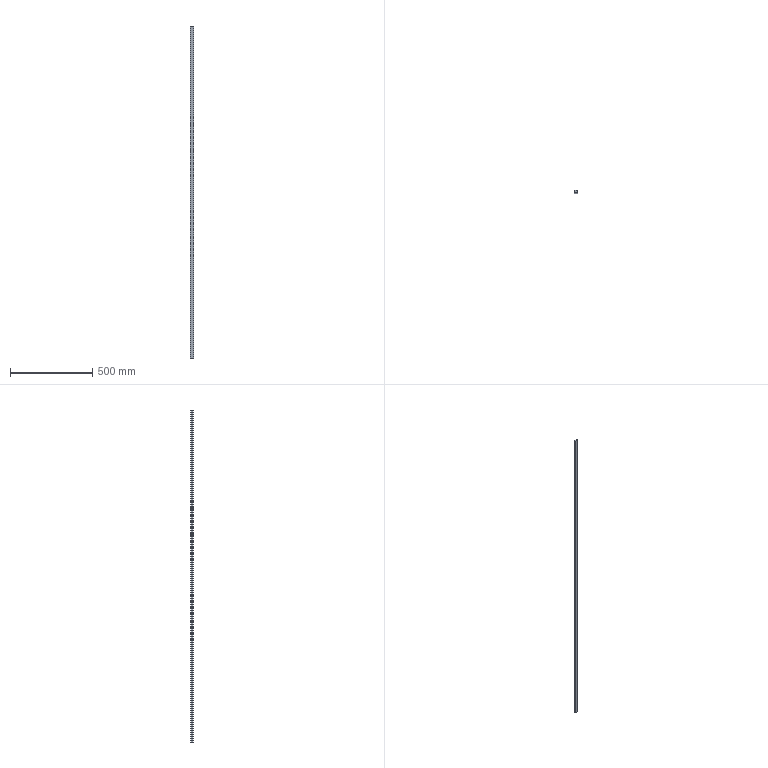Part | STEP file | rail_SX2RZ28_280 | 1 solid | 15 faces | box 20 x 15.5 x 2022 mm | volume 581693 mm3 | plane 10 | cylinder 5 | commonest cylinder face diameters 5 x3 3 x2
STEP:
#1=CARTESIAN_POINT('',(0.,0.,0.));
#2=DIRECTION('',(0.,0.,1.));
#3=DIRECTION('',(1.,0.,0.));
#4=AXIS2_PLACEMENT_3D('',#1,#2,#3);
#5=CARTESIAN_POINT('',(9.062,11.498,1.));
#6=VERTEX_POINT('',#5);
#7=CARTESIAN_POINT('',(9.062,11.498,-2020.5));
#8=VERTEX_POINT('',#7);
#9=CARTESIAN_POINT('',(9.062,11.498,1.));
#10=DIRECTION('',(0.,0.,-1.));
#11=VECTOR('',#10,1.);
#12=LINE('',#9,#11);
#13=CARTESIAN_POINT('',(10.,9.18,1.));
#14=DIRECTION('',(0.,0.,-1.));
#15=DIRECTION('',(-1.,0.,0.));
#16=AXIS2_PLACEMENT_3D('',#13,#14,#15);
#17=CYLINDRICAL_SURFACE('',#16,2.5);
#18=CARTESIAN_POINT('',(1.186,0.));
#19=DIRECTION('',(0.,1.));
#20=VECTOR('',#19,1.);
#21=LINE('',#18,#20);
#22=(GEOMETRIC_REPRESENTATION_CONTEXT(2)PARAMETRIC_REPRESENTATION_CONTEXT()REPRESENTATION_CONTEXT('',''));
#23=DEFINITIONAL_REPRESENTATION('',(#21),#22);
#24=PCURVE('',#17,#23);
#25=CARTESIAN_POINT('',(8.5,12.888,1.));
#26=DIRECTION('',(0.,0.,-1.));
#27=DIRECTION('',(-1.,0.,0.));
#28=AXIS2_PLACEMENT_3D('',#25,#26,#27);
#29=CYLINDRICAL_SURFACE('',#28,1.5);
#30=CARTESIAN_POINT('',(4.328,0.));
#31=DIRECTION('',(0.,1.));
#32=VECTOR('',#31,1.);
#33=LINE('',#30,#32);
#34=(GEOMETRIC_REPRESENTATION_CONTEXT(2)PARAMETRIC_REPRESENTATION_CONTEXT()REPRESENTATION_CONTEXT('',''));
#35=DEFINITIONAL_REPRESENTATION('',(#33),#34);
#36=PCURVE('',#29,#35);
#37=SURFACE_CURVE('',#12,(#24,#36),.PCURVE_S1.);
#38=EDGE_CURVE('',#6,#8,#37,.T.);
#39=ORIENTED_EDGE('',*,*,#38,.T.);
#40=CARTESIAN_POINT('',(7.5,9.18,-2020.5));
#41=VERTEX_POINT('',#40);
#42=CARTESIAN_POINT('',(10.,9.18,-2020.5));
#43=DIRECTION('',(0.,0.,-1.));
#44=DIRECTION('',(-1.,0.,0.));
#45=AXIS2_PLACEMENT_3D('',#42,#43,#44);
#46=CIRCLE('',#45,2.5);
#47=CARTESIAN_POINT('',(0.,2021.5));
#48=DIRECTION('',(1.,0.));
#49=VECTOR('',#48,1.);
#50=LINE('',#47,#49);
#51=(GEOMETRIC_REPRESENTATION_CONTEXT(2)PARAMETRIC_REPRESENTATION_CONTEXT()REPRESENTATION_CONTEXT('',''));
#52=DEFINITIONAL_REPRESENTATION('',(#50),#51);
#53=PCURVE('',#17,#52);
#54=CARTESIAN_POINT('',(10.,9.18,-2020.5));
#55=DIRECTION('',(0.,0.,-1.));
#56=DIRECTION('',(-1.,0.,0.));
#57=AXIS2_PLACEMENT_3D('',#54,#55,#56);
#58=PLANE('',#57);
#59=CARTESIAN_POINT('',(0.,0.));
#60=DIRECTION('',(1.,0.));
#61=AXIS2_PLACEMENT_2D('',#59,#60);
#62=CIRCLE('',#61,2.5);
#63=(GEOMETRIC_REPRESENTATION_CONTEXT(2)PARAMETRIC_REPRESENTATION_CONTEXT()REPRESENTATION_CONTEXT('',''));
#64=DEFINITIONAL_REPRESENTATION('',(#62),#63);
#65=PCURVE('',#58,#64);
#66=SURFACE_CURVE('',#46,(#53,#65),.PCURVE_S1.);
#67=EDGE_CURVE('',#41,#8,#66,.T.);
#68=ORIENTED_EDGE('',*,*,#67,.F.);
#69=CARTESIAN_POINT('',(7.5,9.18,1.));
#70=VERTEX_POINT('',#69);
#71=CARTESIAN_POINT('',(7.5,9.18,1.));
#72=DIRECTION('',(0.,0.,-1.));
#73=VECTOR('',#72,1.);
#74=LINE('',#71,#73);
#75=CARTESIAN_POINT('',(0.,0.));
#76=DIRECTION('',(0.,1.));
#77=VECTOR('',#76,1.);
#78=LINE('',#75,#77);
#79=(GEOMETRIC_REPRESENTATION_CONTEXT(2)PARAMETRIC_REPRESENTATION_CONTEXT()REPRESENTATION_CONTEXT('',''));
#80=DEFINITIONAL_REPRESENTATION('',(#78),#79);
#81=PCURVE('',#17,#80);
#82=CARTESIAN_POINT('',(10.,9.18,1.));
#83=DIRECTION('',(0.,0.,-1.));
#84=DIRECTION('',(-1.,0.,0.));
#85=AXIS2_PLACEMENT_3D('',#82,#83,#84);
#86=CYLINDRICAL_SURFACE('',#85,2.5);
#87=CARTESIAN_POINT('',(6.283,0.));
#88=DIRECTION('',(0.,1.));
#89=VECTOR('',#88,1.);
#90=LINE('',#87,#89);
#91=(GEOMETRIC_REPRESENTATION_CONTEXT(2)PARAMETRIC_REPRESENTATION_CONTEXT()REPRESENTATION_CONTEXT('',''));
#92=DEFINITIONAL_REPRESENTATION('',(#90),#91);
#93=PCURVE('',#86,#92);
#94=SURFACE_CURVE('',#74,(#81,#93),.PCURVE_S1.);
#95=EDGE_CURVE('',#70,#41,#94,.T.);
#96=ORIENTED_EDGE('',*,*,#95,.F.);
#97=CARTESIAN_POINT('',(10.,9.18,1.));
#98=DIRECTION('',(0.,0.,-1.));
#99=DIRECTION('',(-1.,0.,0.));
#100=AXIS2_PLACEMENT_3D('',#97,#98,#99);
#101=CIRCLE('',#100,2.5);
#102=CARTESIAN_POINT('',(0.,0.));
#103=DIRECTION('',(1.,0.));
#104=VECTOR('',#103,1.);
#105=LINE('',#102,#104);
#106=(GEOMETRIC_REPRESENTATION_CONTEXT(2)PARAMETRIC_REPRESENTATION_CONTEXT()REPRESENTATION_CONTEXT('',''));
#107=DEFINITIONAL_REPRESENTATION('',(#105),#106);
#108=PCURVE('',#17,#107);
#109=CARTESIAN_POINT('',(10.,9.18,1.));
#110=DIRECTION('',(0.,0.,-1.));
#111=DIRECTION('',(-1.,0.,0.));
#112=AXIS2_PLACEMENT_3D('',#109,#110,#111);
#113=PLANE('',#112);
#114=CARTESIAN_POINT('',(0.,0.));
#115=DIRECTION('',(1.,0.));
#116=AXIS2_PLACEMENT_2D('',#114,#115);
#117=CIRCLE('',#116,2.5);
#118=(GEOMETRIC_REPRESENTATION_CONTEXT(2)PARAMETRIC_REPRESENTATION_CONTEXT()REPRESENTATION_CONTEXT('',''));
#119=DEFINITIONAL_REPRESENTATION('',(#117),#118);
#120=PCURVE('',#113,#119);
#121=SURFACE_CURVE('',#101,(#108,#120),.PCURVE_S1.);
#122=EDGE_CURVE('',#70,#6,#121,.T.);
#123=ORIENTED_EDGE('',*,*,#122,.T.);
#124=EDGE_LOOP('',(#39,#68,#96,#123));
#125=FACE_BOUND('',#124,.F.);
#126=ADVANCED_FACE('',(#125),#17,.F.);
#127=CARTESIAN_POINT('',(-10.,6.68,1.));
#128=VERTEX_POINT('',#127);
#129=CARTESIAN_POINT('',(-10.,6.68,-2020.5));
#130=VERTEX_POINT('',#129);
#131=CARTESIAN_POINT('',(-10.,6.68,1.));
#132=DIRECTION('',(0.,0.,-1.));
#133=VECTOR('',#132,1.);
#134=LINE('',#131,#133);
#135=CARTESIAN_POINT('',(-10.,6.68,1.));
#136=DIRECTION('',(1.,0.,0.));
#137=DIRECTION('',(0.,0.,-1.));
#138=AXIS2_PLACEMENT_3D('',#135,#136,#137);
#139=PLANE('',#138);
#140=CARTESIAN_POINT('',(0.,0.));
#141=DIRECTION('',(1.,0.));
#142=VECTOR('',#141,1.);
#143=LINE('',#140,#142);
#144=(GEOMETRIC_REPRESENTATION_CONTEXT(2)PARAMETRIC_REPRESENTATION_CONTEXT()REPRESENTATION_CONTEXT('',''));
#145=DEFINITIONAL_REPRESENTATION('',(#143),#144);
#146=PCURVE('',#139,#145);
#147=CARTESIAN_POINT('',(-10.,9.18,1.));
#148=DIRECTION('',(0.,0.,-1.));
#149=DIRECTION('',(-1.,0.,0.));
#150=AXIS2_PLACEMENT_3D('',#147,#148,#149);
#151=CYLINDRICAL_SURFACE('',#150,2.5);
#152=CARTESIAN_POINT('',(4.712,0.));
#153=DIRECTION('',(0.,1.));
#154=VECTOR('',#153,1.);
#155=LINE('',#152,#154);
#156=(GEOMETRIC_REPRESENTATION_CONTEXT(2)PARAMETRIC_REPRESENTATION_CONTEXT()REPRESENTATION_CONTEXT('',''));
#157=DEFINITIONAL_REPRESENTATION('',(#155),#156);
#158=PCURVE('',#151,#157);
#159=SURFACE_CURVE('',#134,(#146,#158),.PCURVE_S1.);
#160=EDGE_CURVE('',#128,#130,#159,.T.);
#161=ORIENTED_EDGE('',*,*,#160,.T.);
#162=CARTESIAN_POINT('',(-10.,0.,-2020.5));
#163=VERTEX_POINT('',#162);
#164=CARTESIAN_POINT('',(-10.,6.68,-2020.5));
#165=DIRECTION('',(0.,-1.,0.));
#166=VECTOR('',#165,1.);
#167=LINE('',#164,#166);
#168=CARTESIAN_POINT('',(2021.5,0.));
#169=DIRECTION('',(0.,-1.));
#170=VECTOR('',#169,1.);
#171=LINE('',#168,#170);
#172=(GEOMETRIC_REPRESENTATION_CONTEXT(2)PARAMETRIC_REPRESENTATION_CONTEXT()REPRESENTATION_CONTEXT('',''));
#173=DEFINITIONAL_REPRESENTATION('',(#171),#172);
#174=PCURVE('',#139,#173);
#175=CARTESIAN_POINT('',(20.,-2.5));
#176=DIRECTION('',(0.,-1.));
#177=VECTOR('',#176,1.);
#178=LINE('',#175,#177);
#179=(GEOMETRIC_REPRESENTATION_CONTEXT(2)PARAMETRIC_REPRESENTATION_CONTEXT()REPRESENTATION_CONTEXT('',''));
#180=DEFINITIONAL_REPRESENTATION('',(#178),#179);
#181=PCURVE('',#58,#180);
#182=SURFACE_CURVE('',#167,(#174,#181),.PCURVE_S1.);
#183=EDGE_CURVE('',#130,#163,#182,.T.);
#184=ORIENTED_EDGE('',*,*,#183,.T.);
#185=CARTESIAN_POINT('',(-10.,0.,1.));
#186=VERTEX_POINT('',#185);
#187=CARTESIAN_POINT('',(-10.,0.,1.));
#188=DIRECTION('',(0.,0.,-1.));
#189=VECTOR('',#188,1.);
#190=LINE('',#187,#189);
#191=CARTESIAN_POINT('',(0.,-6.68));
#192=DIRECTION('',(1.,0.));
#193=VECTOR('',#192,1.);
#194=LINE('',#191,#193);
#195=(GEOMETRIC_REPRESENTATION_CONTEXT(2)PARAMETRIC_REPRESENTATION_CONTEXT()REPRESENTATION_CONTEXT('',''));
#196=DEFINITIONAL_REPRESENTATION('',(#194),#195);
#197=PCURVE('',#139,#196);
#198=CARTESIAN_POINT('',(-10.,0.,1.));
#199=DIRECTION('',(0.,1.,0.));
#200=DIRECTION('',(0.,0.,1.));
#201=AXIS2_PLACEMENT_3D('',#198,#199,#200);
#202=PLANE('',#201);
#203=CARTESIAN_POINT('',(0.,0.));
#204=DIRECTION('',(-1.,0.));
#205=VECTOR('',#204,1.);
#206=LINE('',#203,#205);
#207=(GEOMETRIC_REPRESENTATION_CONTEXT(2)PARAMETRIC_REPRESENTATION_CONTEXT()REPRESENTATION_CONTEXT('',''));
#208=DEFINITIONAL_REPRESENTATION('',(#206),#207);
#209=PCURVE('',#202,#208);
#210=SURFACE_CURVE('',#190,(#197,#209),.PCURVE_S1.);
#211=EDGE_CURVE('',#186,#163,#210,.T.);
#212=ORIENTED_EDGE('',*,*,#211,.F.);
#213=CARTESIAN_POINT('',(-10.,6.68,1.));
#214=DIRECTION('',(0.,-1.,0.));
#215=VECTOR('',#214,1.);
#216=LINE('',#213,#215);
#217=CARTESIAN_POINT('',(0.,0.));
#218=DIRECTION('',(0.,-1.));
#219=VECTOR('',#218,1.);
#220=LINE('',#217,#219);
#221=(GEOMETRIC_REPRESENTATION_CONTEXT(2)PARAMETRIC_REPRESENTATION_CONTEXT()REPRESENTATION_CONTEXT('',''));
#222=DEFINITIONAL_REPRESENTATION('',(#220),#221);
#223=PCURVE('',#139,#222);
#224=CARTESIAN_POINT('',(20.,-2.5));
#225=DIRECTION('',(0.,-1.));
#226=VECTOR('',#225,1.);
#227=LINE('',#224,#226);
#228=(GEOMETRIC_REPRESENTATION_CONTEXT(2)PARAMETRIC_REPRESENTATION_CONTEXT()REPRESENTATION_CONTEXT('',''));
#229=DEFINITIONAL_REPRESENTATION('',(#227),#228);
#230=PCURVE('',#113,#229);
#231=SURFACE_CURVE('',#216,(#223,#230),.PCURVE_S1.);
#232=EDGE_CURVE('',#128,#186,#231,.T.);
#233=ORIENTED_EDGE('',*,*,#232,.F.);
#234=EDGE_LOOP('',(#161,#184,#212,#233));
#235=FACE_BOUND('',#234,.T.);
#236=ADVANCED_FACE('',(#235),#139,.F.);
#237=ORIENTED_EDGE('',*,*,#211,.T.);
#238=CARTESIAN_POINT('',(10.,0.,-2020.5));
#239=VERTEX_POINT('',#238);
#240=CARTESIAN_POINT('',(-10.,0.,-2020.5));
#241=DIRECTION('',(1.,0.,0.));
#242=VECTOR('',#241,1.);
#243=LINE('',#240,#242);
#244=CARTESIAN_POINT('',(-2021.5,0.));
#245=DIRECTION('',(0.,1.));
#246=VECTOR('',#245,1.);
#247=LINE('',#244,#246);
#248=(GEOMETRIC_REPRESENTATION_CONTEXT(2)PARAMETRIC_REPRESENTATION_CONTEXT()REPRESENTATION_CONTEXT('',''));
#249=DEFINITIONAL_REPRESENTATION('',(#247),#248);
#250=PCURVE('',#202,#249);
#251=CARTESIAN_POINT('',(20.,-9.18));
#252=DIRECTION('',(-1.,0.));
#253=VECTOR('',#252,1.);
#254=LINE('',#251,#253);
#255=(GEOMETRIC_REPRESENTATION_CONTEXT(2)PARAMETRIC_REPRESENTATION_CONTEXT()REPRESENTATION_CONTEXT('',''));
#256=DEFINITIONAL_REPRESENTATION('',(#254),#255);
#257=PCURVE('',#58,#256);
#258=SURFACE_CURVE('',#243,(#250,#257),.PCURVE_S1.);
#259=EDGE_CURVE('',#163,#239,#258,.T.);
#260=ORIENTED_EDGE('',*,*,#259,.T.);
#261=CARTESIAN_POINT('',(10.,0.,1.));
#262=VERTEX_POINT('',#261);
#263=CARTESIAN_POINT('',(10.,0.,1.));
#264=DIRECTION('',(0.,0.,-1.));
#265=VECTOR('',#264,1.);
#266=LINE('',#263,#265);
#267=CARTESIAN_POINT('',(0.,20.));
#268=DIRECTION('',(-1.,0.));
#269=VECTOR('',#268,1.);
#270=LINE('',#267,#269);
#271=(GEOMETRIC_REPRESENTATION_CONTEXT(2)PARAMETRIC_REPRESENTATION_CONTEXT()REPRESENTATION_CONTEXT('',''));
#272=DEFINITIONAL_REPRESENTATION('',(#270),#271);
#273=PCURVE('',#202,#272);
#274=CARTESIAN_POINT('',(10.,0.,1.));
#275=DIRECTION('',(-1.,0.,0.));
#276=DIRECTION('',(0.,0.,1.));
#277=AXIS2_PLACEMENT_3D('',#274,#275,#276);
#278=PLANE('',#277);
#279=CARTESIAN_POINT('',(0.,0.));
#280=DIRECTION('',(-1.,0.));
#281=VECTOR('',#280,1.);
#282=LINE('',#279,#281);
#283=(GEOMETRIC_REPRESENTATION_CONTEXT(2)PARAMETRIC_REPRESENTATION_CONTEXT()REPRESENTATION_CONTEXT('',''));
#284=DEFINITIONAL_REPRESENTATION('',(#282),#283);
#285=PCURVE('',#278,#284);
#286=SURFACE_CURVE('',#266,(#273,#285),.PCURVE_S1.);
#287=EDGE_CURVE('',#262,#239,#286,.T.);
#288=ORIENTED_EDGE('',*,*,#287,.F.);
#289=CARTESIAN_POINT('',(-10.,0.,1.));
#290=DIRECTION('',(1.,0.,0.));
#291=VECTOR('',#290,1.);
#292=LINE('',#289,#291);
#293=CARTESIAN_POINT('',(0.,0.));
#294=DIRECTION('',(0.,1.));
#295=VECTOR('',#294,1.);
#296=LINE('',#293,#295);
#297=(GEOMETRIC_REPRESENTATION_CONTEXT(2)PARAMETRIC_REPRESENTATION_CONTEXT()REPRESENTATION_CONTEXT('',''));
#298=DEFINITIONAL_REPRESENTATION('',(#296),#297);
#299=PCURVE('',#202,#298);
#300=CARTESIAN_POINT('',(20.,-9.18));
#301=DIRECTION('',(-1.,0.));
#302=VECTOR('',#301,1.);
#303=LINE('',#300,#302);
#304=(GEOMETRIC_REPRESENTATION_CONTEXT(2)PARAMETRIC_REPRESENTATION_CONTEXT()REPRESENTATION_CONTEXT('',''));
#305=DEFINITIONAL_REPRESENTATION('',(#303),#304);
#306=PCURVE('',#113,#305);
#307=SURFACE_CURVE('',#292,(#299,#306),.PCURVE_S1.);
#308=EDGE_CURVE('',#186,#262,#307,.T.);
#309=ORIENTED_EDGE('',*,*,#308,.F.);
#310=EDGE_LOOP('',(#237,#260,#288,#309));
#311=FACE_BOUND('',#310,.T.);
#312=ADVANCED_FACE('',(#311),#202,.F.);
#313=ORIENTED_EDGE('',*,*,#287,.T.);
#314=CARTESIAN_POINT('',(10.,6.68,-2020.5));
#315=VERTEX_POINT('',#314);
#316=CARTESIAN_POINT('',(10.,0.,-2020.5));
#317=DIRECTION('',(0.,1.,0.));
#318=VECTOR('',#317,1.);
#319=LINE('',#316,#318);
#320=CARTESIAN_POINT('',(-2021.5,0.));
#321=DIRECTION('',(0.,1.));
#322=VECTOR('',#321,1.);
#323=LINE('',#320,#322);
#324=(GEOMETRIC_REPRESENTATION_CONTEXT(2)PARAMETRIC_REPRESENTATION_CONTEXT()REPRESENTATION_CONTEXT('',''));
#325=DEFINITIONAL_REPRESENTATION('',(#323),#324);
#326=PCURVE('',#278,#325);
#327=CARTESIAN_POINT('',(0.,-9.18));
#328=DIRECTION('',(0.,1.));
#329=VECTOR('',#328,1.);
#330=LINE('',#327,#329);
#331=(GEOMETRIC_REPRESENTATION_CONTEXT(2)PARAMETRIC_REPRESENTATION_CONTEXT()REPRESENTATION_CONTEXT('',''));
#332=DEFINITIONAL_REPRESENTATION('',(#330),#331);
#333=PCURVE('',#58,#332);
#334=SURFACE_CURVE('',#319,(#326,#333),.PCURVE_S1.);
#335=EDGE_CURVE('',#239,#315,#334,.T.);
#336=ORIENTED_EDGE('',*,*,#335,.T.);
#337=CARTESIAN_POINT('',(10.,6.68,1.));
#338=VERTEX_POINT('',#337);
#339=CARTESIAN_POINT('',(10.,6.68,1.));
#340=DIRECTION('',(0.,0.,-1.));
#341=VECTOR('',#340,1.);
#342=LINE('',#339,#341);
#343=CARTESIAN_POINT('',(0.,6.68));
#344=DIRECTION('',(-1.,0.));
#345=VECTOR('',#344,1.);
#346=LINE('',#343,#345);
#347=(GEOMETRIC_REPRESENTATION_CONTEXT(2)PARAMETRIC_REPRESENTATION_CONTEXT()REPRESENTATION_CONTEXT('',''));
#348=DEFINITIONAL_REPRESENTATION('',(#346),#347);
#349=PCURVE('',#278,#348);
#350=CARTESIAN_POINT('',(4.712,0.));
#351=DIRECTION('',(0.,1.));
#352=VECTOR('',#351,1.);
#353=LINE('',#350,#352);
#354=(GEOMETRIC_REPRESENTATION_CONTEXT(2)PARAMETRIC_REPRESENTATION_CONTEXT()REPRESENTATION_CONTEXT('',''));
#355=DEFINITIONAL_REPRESENTATION('',(#353),#354);
#356=PCURVE('',#86,#355);
#357=SURFACE_CURVE('',#342,(#349,#356),.PCURVE_S1.);
#358=EDGE_CURVE('',#338,#315,#357,.T.);
#359=ORIENTED_EDGE('',*,*,#358,.F.);
#360=CARTESIAN_POINT('',(10.,0.,1.));
#361=DIRECTION('',(0.,1.,0.));
#362=VECTOR('',#361,1.);
#363=LINE('',#360,#362);
#364=CARTESIAN_POINT('',(0.,0.));
#365=DIRECTION('',(0.,1.));
#366=VECTOR('',#365,1.);
#367=LINE('',#364,#366);
#368=(GEOMETRIC_REPRESENTATION_CONTEXT(2)PARAMETRIC_REPRESENTATION_CONTEXT()REPRESENTATION_CONTEXT('',''));
#369=DEFINITIONAL_REPRESENTATION('',(#367),#368);
#370=PCURVE('',#278,#369);
#371=CARTESIAN_POINT('',(0.,-9.18));
#372=DIRECTION('',(0.,1.));
#373=VECTOR('',#372,1.);
#374=LINE('',#371,#373);
#375=(GEOMETRIC_REPRESENTATION_CONTEXT(2)PARAMETRIC_REPRESENTATION_CONTEXT()REPRESENTATION_CONTEXT('',''));
#376=DEFINITIONAL_REPRESENTATION('',(#374),#375);
#377=PCURVE('',#113,#376);
#378=SURFACE_CURVE('',#363,(#370,#377),.PCURVE_S1.);
#379=EDGE_CURVE('',#262,#338,#378,.T.);
#380=ORIENTED_EDGE('',*,*,#379,.F.);
#381=EDGE_LOOP('',(#313,#336,#359,#380));
#382=FACE_BOUND('',#381,.T.);
#383=ADVANCED_FACE('',(#382),#278,.F.);
#384=CARTESIAN_POINT('',(10.,9.18,-2020.5));
#385=DIRECTION('',(0.,0.,-1.));
#386=DIRECTION('',(-1.,0.,0.));
#387=AXIS2_PLACEMENT_3D('',#384,#385,#386);
#388=CIRCLE('',#387,2.5);
#389=CARTESIAN_POINT('',(0.,2021.5));
#390=DIRECTION('',(1.,0.));
#391=VECTOR('',#390,1.);
#392=LINE('',#389,#391);
#393=(GEOMETRIC_REPRESENTATION_CONTEXT(2)PARAMETRIC_REPRESENTATION_CONTEXT()REPRESENTATION_CONTEXT('',''));
#394=DEFINITIONAL_REPRESENTATION('',(#392),#393);
#395=PCURVE('',#86,#394);
#396=CARTESIAN_POINT('',(0.,0.));
#397=DIRECTION('',(1.,0.));
#398=AXIS2_PLACEMENT_2D('',#396,#397);
#399=CIRCLE('',#398,2.5);
#400=(GEOMETRIC_REPRESENTATION_CONTEXT(2)PARAMETRIC_REPRESENTATION_CONTEXT()REPRESENTATION_CONTEXT('',''));
#401=DEFINITIONAL_REPRESENTATION('',(#399),#400);
#402=PCURVE('',#58,#401);
#403=SURFACE_CURVE('',#388,(#395,#402),.PCURVE_S1.);
#404=EDGE_CURVE('',#315,#41,#403,.T.);
#405=ORIENTED_EDGE('',*,*,#404,.F.);
#406=ORIENTED_EDGE('',*,*,#358,.F.);
#407=CARTESIAN_POINT('',(10.,9.18,1.));
#408=DIRECTION('',(0.,0.,-1.));
#409=DIRECTION('',(-1.,0.,0.));
#410=AXIS2_PLACEMENT_3D('',#407,#408,#409);
#411=CIRCLE('',#410,2.5);
#412=CARTESIAN_POINT('',(0.,0.));
#413=DIRECTION('',(1.,0.));
#414=VECTOR('',#413,1.);
#415=LINE('',#412,#414);
#416=(GEOMETRIC_REPRESENTATION_CONTEXT(2)PARAMETRIC_REPRESENTATION_CONTEXT()REPRESENTATION_CONTEXT('',''));
#417=DEFINITIONAL_REPRESENTATION('',(#415),#416);
#418=PCURVE('',#86,#417);
#419=CARTESIAN_POINT('',(0.,0.));
#420=DIRECTION('',(1.,0.));
#421=AXIS2_PLACEMENT_2D('',#419,#420);
#422=CIRCLE('',#421,2.5);
#423=(GEOMETRIC_REPRESENTATION_CONTEXT(2)PARAMETRIC_REPRESENTATION_CONTEXT()REPRESENTATION_CONTEXT('',''));
#424=DEFINITIONAL_REPRESENTATION('',(#422),#423);
#425=PCURVE('',#113,#424);
#426=SURFACE_CURVE('',#411,(#418,#425),.PCURVE_S1.);
#427=EDGE_CURVE('',#338,#70,#426,.T.);
#428=ORIENTED_EDGE('',*,*,#427,.T.);
#429=ORIENTED_EDGE('',*,*,#95,.T.);
#430=EDGE_LOOP('',(#405,#406,#428,#429));
#431=FACE_BOUND('',#430,.F.);
#432=ADVANCED_FACE('',(#431),#86,.F.);
#433=ORIENTED_EDGE('',*,*,#38,.T.);
#434=CARTESIAN_POINT('',(10.,12.888,-2020.5));
#435=VERTEX_POINT('',#434);
#436=CARTESIAN_POINT('',(8.5,12.888,-2020.5));
#437=DIRECTION('',(0.,0.,1.));
#438=DIRECTION('',(1.,0.,0.));
#439=AXIS2_PLACEMENT_3D('',#436,#437,#438);
#440=CIRCLE('',#439,1.5);
#441=CARTESIAN_POINT('',(9.425,2021.5));
#442=DIRECTION('',(-1.,0.));
#443=VECTOR('',#442,1.);
#444=LINE('',#441,#443);
#445=(GEOMETRIC_REPRESENTATION_CONTEXT(2)PARAMETRIC_REPRESENTATION_CONTEXT()REPRESENTATION_CONTEXT('',''));
#446=DEFINITIONAL_REPRESENTATION('',(#444),#445);
#447=PCURVE('',#29,#446);
#448=CARTESIAN_POINT('',(0.,3.708));
#449=CARTESIAN_POINT('',(0.,6.306));
#450=CARTESIAN_POINT('',(2.25,5.007));
#451=CARTESIAN_POINT('',(4.5,3.708));
#452=CARTESIAN_POINT('',(2.25,2.409));
#453=CARTESIAN_POINT('',(0.,1.11));
#454=CARTESIAN_POINT('',(0.,3.708));
#455=(BOUNDED_CURVE()B_SPLINE_CURVE(2,(#448,#449,#450,#451,#452,#453,#454),.UNSPECIFIED.,.T.,.F.)B_SPLINE_CURVE_WITH_KNOTS((1,2,2,2,2,1),(-2.094,0.,2.094,4.189,6.283,8.378),.UNSPECIFIED.)CURVE()GEOMETRIC_REPRESENTATION_ITEM()RATIONAL_B_SPLINE_CURVE((1.,0.5,1.,0.5,1.,0.5,1.))REPRESENTATION_ITEM(''));
#456=(GEOMETRIC_REPRESENTATION_CONTEXT(2)PARAMETRIC_REPRESENTATION_CONTEXT()REPRESENTATION_CONTEXT('',''));
#457=DEFINITIONAL_REPRESENTATION('',(#455),#456);
#458=PCURVE('',#58,#457);
#459=SURFACE_CURVE('',#440,(#447,#458),.PCURVE_S1.);
#460=EDGE_CURVE('',#8,#435,#459,.T.);
#461=ORIENTED_EDGE('',*,*,#460,.T.);
#462=CARTESIAN_POINT('',(10.,12.888,1.));
#463=VERTEX_POINT('',#462);
#464=CARTESIAN_POINT('',(10.,12.888,1.));
#465=DIRECTION('',(0.,0.,-1.));
#466=VECTOR('',#465,1.);
#467=LINE('',#464,#466);
#468=CARTESIAN_POINT('',(3.142,0.));
#469=DIRECTION('',(0.,1.));
#470=VECTOR('',#469,1.);
#471=LINE('',#468,#470);
#472=(GEOMETRIC_REPRESENTATION_CONTEXT(2)PARAMETRIC_REPRESENTATION_CONTEXT()REPRESENTATION_CONTEXT('',''));
#473=DEFINITIONAL_REPRESENTATION('',(#471),#472);
#474=PCURVE('',#29,#473);
#475=CARTESIAN_POINT('',(10.,12.888,1.));
#476=DIRECTION('',(-1.,0.,0.));
#477=DIRECTION('',(0.,0.,1.));
#478=AXIS2_PLACEMENT_3D('',#475,#476,#477);
#479=PLANE('',#478);
#480=CARTESIAN_POINT('',(0.,0.));
#481=DIRECTION('',(-1.,0.));
#482=VECTOR('',#481,1.);
#483=LINE('',#480,#482);
#484=(GEOMETRIC_REPRESENTATION_CONTEXT(2)PARAMETRIC_REPRESENTATION_CONTEXT()REPRESENTATION_CONTEXT('',''));
#485=DEFINITIONAL_REPRESENTATION('',(#483),#484);
#486=PCURVE('',#479,#485);
#487=SURFACE_CURVE('',#467,(#474,#486),.PCURVE_S1.);
#488=EDGE_CURVE('',#463,#435,#487,.T.);
#489=ORIENTED_EDGE('',*,*,#488,.F.);
#490=CARTESIAN_POINT('',(8.5,12.888,1.));
#491=DIRECTION('',(0.,0.,1.));
#492=DIRECTION('',(1.,0.,0.));
#493=AXIS2_PLACEMENT_3D('',#490,#491,#492);
#494=CIRCLE('',#493,1.5);
#495=CARTESIAN_POINT('',(9.425,0.));
#496=DIRECTION('',(-1.,0.));
#497=VECTOR('',#496,1.);
#498=LINE('',#495,#497);
#499=(GEOMETRIC_REPRESENTATION_CONTEXT(2)PARAMETRIC_REPRESENTATION_CONTEXT()REPRESENTATION_CONTEXT('',''));
#500=DEFINITIONAL_REPRESENTATION('',(#498),#499);
#501=PCURVE('',#29,#500);
#502=CARTESIAN_POINT('',(0.,3.708));
#503=CARTESIAN_POINT('',(0.,6.306));
#504=CARTESIAN_POINT('',(2.25,5.007));
#505=CARTESIAN_POINT('',(4.5,3.708));
#506=CARTESIAN_POINT('',(2.25,2.409));
#507=CARTESIAN_POINT('',(0.,1.11));
#508=CARTESIAN_POINT('',(0.,3.708));
#509=(BOUNDED_CURVE()B_SPLINE_CURVE(2,(#502,#503,#504,#505,#506,#507,#508),.UNSPECIFIED.,.T.,.F.)B_SPLINE_CURVE_WITH_KNOTS((1,2,2,2,2,1),(-2.094,0.,2.094,4.189,6.283,8.378),.UNSPECIFIED.)CURVE()GEOMETRIC_REPRESENTATION_ITEM()RATIONAL_B_SPLINE_CURVE((1.,0.5,1.,0.5,1.,0.5,1.))REPRESENTATION_ITEM(''));
#510=(GEOMETRIC_REPRESENTATION_CONTEXT(2)PARAMETRIC_REPRESENTATION_CONTEXT()REPRESENTATION_CONTEXT('',''));
#511=DEFINITIONAL_REPRESENTATION('',(#509),#510);
#512=PCURVE('',#113,#511);
#513=SURFACE_CURVE('',#494,(#501,#512),.PCURVE_S1.);
#514=EDGE_CURVE('',#6,#463,#513,.T.);
#515=ORIENTED_EDGE('',*,*,#514,.F.);
#516=EDGE_LOOP('',(#433,#461,#489,#515));
#517=FACE_BOUND('',#516,.T.);
#518=ADVANCED_FACE('',(#517),#29,.T.);
#519=ORIENTED_EDGE('',*,*,#488,.T.);
#520=CARTESIAN_POINT('',(10.,14.043,-2020.5));
#521=VERTEX_POINT('',#520);
#522=CARTESIAN_POINT('',(10.,12.888,-2020.5));
#523=DIRECTION('',(0.,1.,0.));
#524=VECTOR('',#523,1.);
#525=LINE('',#522,#524);
#526=CARTESIAN_POINT('',(-2021.5,0.));
#527=DIRECTION('',(0.,1.));
#528=VECTOR('',#527,1.);
#529=LINE('',#526,#528);
#530=(GEOMETRIC_REPRESENTATION_CONTEXT(2)PARAMETRIC_REPRESENTATION_CONTEXT()REPRESENTATION_CONTEXT('',''));
#531=DEFINITIONAL_REPRESENTATION('',(#529),#530);
#532=PCURVE('',#479,#531);
#533=CARTESIAN_POINT('',(0.,3.708));
#534=DIRECTION('',(0.,1.));
#535=VECTOR('',#534,1.);
#536=LINE('',#533,#535);
#537=(GEOMETRIC_REPRESENTATION_CONTEXT(2)PARAMETRIC_REPRESENTATION_CONTEXT()REPRESENTATION_CONTEXT('',''));
#538=DEFINITIONAL_REPRESENTATION('',(#536),#537);
#539=PCURVE('',#58,#538);
#540=SURFACE_CURVE('',#525,(#532,#539),.PCURVE_S1.);
#541=EDGE_CURVE('',#435,#521,#540,.T.);
#542=ORIENTED_EDGE('',*,*,#541,.T.);
#543=CARTESIAN_POINT('',(10.,14.043,1.));
#544=VERTEX_POINT('',#543);
#545=CARTESIAN_POINT('',(10.,14.043,1.));
#546=DIRECTION('',(0.,0.,-1.));
#547=VECTOR('',#546,1.);
#548=LINE('',#545,#547);
#549=CARTESIAN_POINT('',(0.,1.155));
#550=DIRECTION('',(-1.,0.));
#551=VECTOR('',#550,1.);
#552=LINE('',#549,#551);
#553=(GEOMETRIC_REPRESENTATION_CONTEXT(2)PARAMETRIC_REPRESENTATION_CONTEXT()REPRESENTATION_CONTEXT('',''));
#554=DEFINITIONAL_REPRESENTATION('',(#552),#553);
#555=PCURVE('',#479,#554);
#556=CARTESIAN_POINT('',(10.,14.043,1.));
#557=DIRECTION('',(-0.7071,-0.7071,0.));
#558=DIRECTION('',(0.7071,-0.7071,0.));
#559=AXIS2_PLACEMENT_3D('',#556,#557,#558);
#560=PLANE('',#559);
#561=CARTESIAN_POINT('',(0.,0.));
#562=DIRECTION('',(0.,-1.));
#563=VECTOR('',#562,1.);
#564=LINE('',#561,#563);
#565=(GEOMETRIC_REPRESENTATION_CONTEXT(2)PARAMETRIC_REPRESENTATION_CONTEXT()REPRESENTATION_CONTEXT('',''));
#566=DEFINITIONAL_REPRESENTATION('',(#564),#565);
#567=PCURVE('',#560,#566);
#568=SURFACE_CURVE('',#548,(#555,#567),.PCURVE_S1.);
#569=EDGE_CURVE('',#544,#521,#568,.T.);
#570=ORIENTED_EDGE('',*,*,#569,.F.);
#571=CARTESIAN_POINT('',(10.,12.888,1.));
#572=DIRECTION('',(0.,1.,0.));
#573=VECTOR('',#572,1.);
#574=LINE('',#571,#573);
#575=CARTESIAN_POINT('',(0.,0.));
#576=DIRECTION('',(0.,1.));
#577=VECTOR('',#576,1.);
#578=LINE('',#575,#577);
#579=(GEOMETRIC_REPRESENTATION_CONTEXT(2)PARAMETRIC_REPRESENTATION_CONTEXT()REPRESENTATION_CONTEXT('',''));
#580=DEFINITIONAL_REPRESENTATION('',(#578),#579);
#581=PCURVE('',#479,#580);
#582=CARTESIAN_POINT('',(0.,3.708));
#583=DIRECTION('',(0.,1.));
#584=VECTOR('',#583,1.);
#585=LINE('',#582,#584);
#586=(GEOMETRIC_REPRESENTATION_CONTEXT(2)PARAMETRIC_REPRESENTATION_CONTEXT()REPRESENTATION_CONTEXT('',''));
#587=DEFINITIONAL_REPRESENTATION('',(#585),#586);
#588=PCURVE('',#113,#587);
#589=SURFACE_CURVE('',#574,(#581,#588),.PCURVE_S1.);
#590=EDGE_CURVE('',#463,#544,#589,.T.);
#591=ORIENTED_EDGE('',*,*,#590,.F.);
#592=EDGE_LOOP('',(#519,#542,#570,#591));
#593=FACE_BOUND('',#592,.T.);
#594=ADVANCED_FACE('',(#593),#479,.F.);
#595=ORIENTED_EDGE('',*,*,#569,.T.);
#596=CARTESIAN_POINT('',(8.543,15.5,-2020.5));
#597=VERTEX_POINT('',#596);
#598=CARTESIAN_POINT('',(10.,14.043,-2020.5));
#599=DIRECTION('',(-0.7071,0.7071,0.));
#600=VECTOR('',#599,1.);
#601=LINE('',#598,#600);
#602=CARTESIAN_POINT('',(0.,-2021.5));
#603=DIRECTION('',(-1.,0.));
#604=VECTOR('',#603,1.);
#605=LINE('',#602,#604);
#606=(GEOMETRIC_REPRESENTATION_CONTEXT(2)PARAMETRIC_REPRESENTATION_CONTEXT()REPRESENTATION_CONTEXT('',''));
#607=DEFINITIONAL_REPRESENTATION('',(#605),#606);
#608=PCURVE('',#560,#607);
#609=CARTESIAN_POINT('',(0.,4.863));
#610=DIRECTION('',(0.7071,0.7071));
#611=VECTOR('',#610,1.);
#612=LINE('',#609,#611);
#613=(GEOMETRIC_REPRESENTATION_CONTEXT(2)PARAMETRIC_REPRESENTATION_CONTEXT()REPRESENTATION_CONTEXT('',''));
#614=DEFINITIONAL_REPRESENTATION('',(#612),#613);
#615=PCURVE('',#58,#614);
#616=SURFACE_CURVE('',#601,(#608,#615),.PCURVE_S1.);
#617=EDGE_CURVE('',#521,#597,#616,.T.);
#618=ORIENTED_EDGE('',*,*,#617,.T.);
#619=CARTESIAN_POINT('',(8.543,15.5,1.));
#620=VERTEX_POINT('',#619);
#621=CARTESIAN_POINT('',(8.543,15.5,1.));
#622=DIRECTION('',(0.,0.,-1.));
#623=VECTOR('',#622,1.);
#624=LINE('',#621,#623);
#625=CARTESIAN_POINT('',(-2.06,0.));
#626=DIRECTION('',(0.,-1.));
#627=VECTOR('',#626,1.);
#628=LINE('',#625,#627);
#629=(GEOMETRIC_REPRESENTATION_CONTEXT(2)PARAMETRIC_REPRESENTATION_CONTEXT()REPRESENTATION_CONTEXT('',''));
#630=DEFINITIONAL_REPRESENTATION('',(#628),#629);
#631=PCURVE('',#560,#630);
#632=CARTESIAN_POINT('',(8.543,15.5,1.));
#633=DIRECTION('',(0.,-1.,0.));
#634=DIRECTION('',(0.,0.,-1.));
#635=AXIS2_PLACEMENT_3D('',#632,#633,#634);
#636=PLANE('',#635);
#637=CARTESIAN_POINT('',(0.,0.));
#638=DIRECTION('',(1.,0.));
#639=VECTOR('',#638,1.);
#640=LINE('',#637,#639);
#641=(GEOMETRIC_REPRESENTATION_CONTEXT(2)PARAMETRIC_REPRESENTATION_CONTEXT()REPRESENTATION_CONTEXT('',''));
#642=DEFINITIONAL_REPRESENTATION('',(#640),#641);
#643=PCURVE('',#636,#642);
#644=SURFACE_CURVE('',#624,(#631,#643),.PCURVE_S1.);
#645=EDGE_CURVE('',#620,#597,#644,.T.);
#646=ORIENTED_EDGE('',*,*,#645,.F.);
#647=CARTESIAN_POINT('',(10.,14.043,1.));
#648=DIRECTION('',(-0.7071,0.7071,0.));
#649=VECTOR('',#648,1.);
#650=LINE('',#647,#649);
#651=CARTESIAN_POINT('',(0.,0.));
#652=DIRECTION('',(-1.,0.));
#653=VECTOR('',#652,1.);
#654=LINE('',#651,#653);
#655=(GEOMETRIC_REPRESENTATION_CONTEXT(2)PARAMETRIC_REPRESENTATION_CONTEXT()REPRESENTATION_CONTEXT('',''));
#656=DEFINITIONAL_REPRESENTATION('',(#654),#655);
#657=PCURVE('',#560,#656);
#658=CARTESIAN_POINT('',(0.,4.863));
#659=DIRECTION('',(0.7071,0.7071));
#660=VECTOR('',#659,1.);
#661=LINE('',#658,#660);
#662=(GEOMETRIC_REPRESENTATION_CONTEXT(2)PARAMETRIC_REPRESENTATION_CONTEXT()REPRESENTATION_CONTEXT('',''));
#663=DEFINITIONAL_REPRESENTATION('',(#661),#662);
#664=PCURVE('',#113,#663);
#665=SURFACE_CURVE('',#650,(#657,#664),.PCURVE_S1.);
#666=EDGE_CURVE('',#544,#620,#665,.T.);
#667=ORIENTED_EDGE('',*,*,#666,.F.);
#668=EDGE_LOOP('',(#595,#618,#646,#667));
#669=FACE_BOUND('',#668,.T.);
#670=ADVANCED_FACE('',(#669),#560,.F.);
#671=ORIENTED_EDGE('',*,*,#645,.T.);
#672=CARTESIAN_POINT('',(-8.543,15.5,-2020.5));
#673=VERTEX_POINT('',#672);
#674=CARTESIAN_POINT('',(8.543,15.5,-2020.5));
#675=DIRECTION('',(-1.,0.,0.));
#676=VECTOR('',#675,1.);
#677=LINE('',#674,#676);
#678=CARTESIAN_POINT('',(2021.5,0.));
#679=DIRECTION('',(0.,-1.));
#680=VECTOR('',#679,1.);
#681=LINE('',#678,#680);
#682=(GEOMETRIC_REPRESENTATION_CONTEXT(2)PARAMETRIC_REPRESENTATION_CONTEXT()REPRESENTATION_CONTEXT('',''));
#683=DEFINITIONAL_REPRESENTATION('',(#681),#682);
#684=PCURVE('',#636,#683);
#685=CARTESIAN_POINT('',(1.457,6.32));
#686=DIRECTION('',(1.,0.));
#687=VECTOR('',#686,1.);
#688=LINE('',#685,#687);
#689=(GEOMETRIC_REPRESENTATION_CONTEXT(2)PARAMETRIC_REPRESENTATION_CONTEXT()REPRESENTATION_CONTEXT('',''));
#690=DEFINITIONAL_REPRESENTATION('',(#688),#689);
#691=PCURVE('',#58,#690);
#692=SURFACE_CURVE('',#677,(#684,#691),.PCURVE_S1.);
#693=EDGE_CURVE('',#597,#673,#692,.T.);
#694=ORIENTED_EDGE('',*,*,#693,.T.);
#695=CARTESIAN_POINT('',(-8.543,15.5,1.));
#696=VERTEX_POINT('',#695);
#697=CARTESIAN_POINT('',(-8.543,15.5,1.));
#698=DIRECTION('',(0.,0.,-1.));
#699=VECTOR('',#698,1.);
#700=LINE('',#697,#699);
#701=CARTESIAN_POINT('',(0.,-17.087));
#702=DIRECTION('',(1.,0.));
#703=VECTOR('',#702,1.);
#704=LINE('',#701,#703);
#705=(GEOMETRIC_REPRESENTATION_CONTEXT(2)PARAMETRIC_REPRESENTATION_CONTEXT()REPRESENTATION_CONTEXT('',''));
#706=DEFINITIONAL_REPRESENTATION('',(#704),#705);
#707=PCURVE('',#636,#706);
#708=CARTESIAN_POINT('',(-8.543,15.5,1.));
#709=DIRECTION('',(0.7071,-0.7071,0.));
#710=DIRECTION('',(0.7071,0.7071,0.));
#711=AXIS2_PLACEMENT_3D('',#708,#709,#710);
#712=PLANE('',#711);
#713=CARTESIAN_POINT('',(0.,0.));
#714=DIRECTION('',(0.,-1.));
#715=VECTOR('',#714,1.);
#716=LINE('',#713,#715);
#717=(GEOMETRIC_REPRESENTATION_CONTEXT(2)PARAMETRIC_REPRESENTATION_CONTEXT()REPRESENTATION_CONTEXT('',''));
#718=DEFINITIONAL_REPRESENTATION('',(#716),#717);
#719=PCURVE('',#712,#718);
#720=SURFACE_CURVE('',#700,(#707,#719),.PCURVE_S1.);
#721=EDGE_CURVE('',#696,#673,#720,.T.);
#722=ORIENTED_EDGE('',*,*,#721,.F.);
#723=CARTESIAN_POINT('',(8.543,15.5,1.));
#724=DIRECTION('',(-1.,0.,0.));
#725=VECTOR('',#724,1.);
#726=LINE('',#723,#725);
#727=CARTESIAN_POINT('',(0.,0.));
#728=DIRECTION('',(0.,-1.));
#729=VECTOR('',#728,1.);
#730=LINE('',#727,#729);
#731=(GEOMETRIC_REPRESENTATION_CONTEXT(2)PARAMETRIC_REPRESENTATION_CONTEXT()REPRESENTATION_CONTEXT('',''));
#732=DEFINITIONAL_REPRESENTATION('',(#730),#731);
#733=PCURVE('',#636,#732);
#734=CARTESIAN_POINT('',(1.457,6.32));
#735=DIRECTION('',(1.,0.));
#736=VECTOR('',#735,1.);
#737=LINE('',#734,#736);
#738=(GEOMETRIC_REPRESENTATION_CONTEXT(2)PARAMETRIC_REPRESENTATION_CONTEXT()REPRESENTATION_CONTEXT('',''));
#739=DEFINITIONAL_REPRESENTATION('',(#737),#738);
#740=PCURVE('',#113,#739);
#741=SURFACE_CURVE('',#726,(#733,#740),.PCURVE_S1.);
#742=EDGE_CURVE('',#620,#696,#741,.T.);
#743=ORIENTED_EDGE('',*,*,#742,.F.);
#744=EDGE_LOOP('',(#671,#694,#722,#743));
#745=FACE_BOUND('',#744,.T.);
#746=ADVANCED_FACE('',(#745),#636,.F.);
#747=ORIENTED_EDGE('',*,*,#721,.T.);
#748=CARTESIAN_POINT('',(-10.,14.043,-2020.5));
#749=VERTEX_POINT('',#748);
#750=CARTESIAN_POINT('',(-8.543,15.5,-2020.5));
#751=DIRECTION('',(-0.7071,-0.7071,0.));
#752=VECTOR('',#751,1.);
#753=LINE('',#750,#752);
#754=CARTESIAN_POINT('',(0.,-2021.5));
#755=DIRECTION('',(-1.,0.));
#756=VECTOR('',#755,1.);
#757=LINE('',#754,#756);
#758=(GEOMETRIC_REPRESENTATION_CONTEXT(2)PARAMETRIC_REPRESENTATION_CONTEXT()REPRESENTATION_CONTEXT('',''));
#759=DEFINITIONAL_REPRESENTATION('',(#757),#758);
#760=PCURVE('',#712,#759);
#761=CARTESIAN_POINT('',(18.543,6.32));
#762=DIRECTION('',(0.7071,-0.7071));
#763=VECTOR('',#762,1.);
#764=LINE('',#761,#763);
#765=(GEOMETRIC_REPRESENTATION_CONTEXT(2)PARAMETRIC_REPRESENTATION_CONTEXT()REPRESENTATION_CONTEXT('',''));
#766=DEFINITIONAL_REPRESENTATION('',(#764),#765);
#767=PCURVE('',#58,#766);
#768=SURFACE_CURVE('',#753,(#760,#767),.PCURVE_S1.);
#769=EDGE_CURVE('',#673,#749,#768,.T.);
#770=ORIENTED_EDGE('',*,*,#769,.T.);
#771=CARTESIAN_POINT('',(-10.,14.043,1.));
#772=VERTEX_POINT('',#771);
#773=CARTESIAN_POINT('',(-10.,14.043,1.));
#774=DIRECTION('',(0.,0.,-1.));
#775=VECTOR('',#774,1.);
#776=LINE('',#773,#775);
#777=CARTESIAN_POINT('',(-2.06,0.));
#778=DIRECTION('',(0.,-1.));
#779=VECTOR('',#778,1.);
#780=LINE('',#777,#779);
#781=(GEOMETRIC_REPRESENTATION_CONTEXT(2)PARAMETRIC_REPRESENTATION_CONTEXT()REPRESENTATION_CONTEXT('',''));
#782=DEFINITIONAL_REPRESENTATION('',(#780),#781);
#783=PCURVE('',#712,#782);
#784=CARTESIAN_POINT('',(-10.,14.043,1.));
#785=DIRECTION('',(1.,0.,0.));
#786=DIRECTION('',(0.,0.,-1.));
#787=AXIS2_PLACEMENT_3D('',#784,#785,#786);
#788=PLANE('',#787);
#789=CARTESIAN_POINT('',(0.,0.));
#790=DIRECTION('',(1.,0.));
#791=VECTOR('',#790,1.);
#792=LINE('',#789,#791);
#793=(GEOMETRIC_REPRESENTATION_CONTEXT(2)PARAMETRIC_REPRESENTATION_CONTEXT()REPRESENTATION_CONTEXT('',''));
#794=DEFINITIONAL_REPRESENTATION('',(#792),#793);
#795=PCURVE('',#788,#794);
#796=SURFACE_CURVE('',#776,(#783,#795),.PCURVE_S1.);
#797=EDGE_CURVE('',#772,#749,#796,.T.);
#798=ORIENTED_EDGE('',*,*,#797,.F.);
#799=CARTESIAN_POINT('',(-8.543,15.5,1.));
#800=DIRECTION('',(-0.7071,-0.7071,0.));
#801=VECTOR('',#800,1.);
#802=LINE('',#799,#801);
#803=CARTESIAN_POINT('',(0.,0.));
#804=DIRECTION('',(-1.,0.));
#805=VECTOR('',#804,1.);
#806=LINE('',#803,#805);
#807=(GEOMETRIC_REPRESENTATION_CONTEXT(2)PARAMETRIC_REPRESENTATION_CONTEXT()REPRESENTATION_CONTEXT('',''));
#808=DEFINITIONAL_REPRESENTATION('',(#806),#807);
#809=PCURVE('',#712,#808);
#810=CARTESIAN_POINT('',(18.543,6.32));
#811=DIRECTION('',(0.7071,-0.7071));
#812=VECTOR('',#811,1.);
#813=LINE('',#810,#812);
#814=(GEOMETRIC_REPRESENTATION_CONTEXT(2)PARAMETRIC_REPRESENTATION_CONTEXT()REPRESENTATION_CONTEXT('',''));
#815=DEFINITIONAL_REPRESENTATION('',(#813),#814);
#816=PCURVE('',#113,#815);
#817=SURFACE_CURVE('',#802,(#809,#816),.PCURVE_S1.);
#818=EDGE_CURVE('',#696,#772,#817,.T.);
#819=ORIENTED_EDGE('',*,*,#818,.F.);
#820=EDGE_LOOP('',(#747,#770,#798,#819));
#821=FACE_BOUND('',#820,.T.);
#822=ADVANCED_FACE('',(#821),#712,.F.);
#823=ORIENTED_EDGE('',*,*,#797,.T.);
#824=CARTESIAN_POINT('',(-10.,12.888,-2020.5));
#825=VERTEX_POINT('',#824);
#826=CARTESIAN_POINT('',(-10.,14.043,-2020.5));
#827=DIRECTION('',(0.,-1.,0.));
#828=VECTOR('',#827,1.);
#829=LINE('',#826,#828);
#830=CARTESIAN_POINT('',(2021.5,0.));
#831=DIRECTION('',(0.,-1.));
#832=VECTOR('',#831,1.);
#833=LINE('',#830,#832);
#834=(GEOMETRIC_REPRESENTATION_CONTEXT(2)PARAMETRIC_REPRESENTATION_CONTEXT()REPRESENTATION_CONTEXT('',''));
#835=DEFINITIONAL_REPRESENTATION('',(#833),#834);
#836=PCURVE('',#788,#835);
#837=CARTESIAN_POINT('',(20.,4.863));
#838=DIRECTION('',(0.,-1.));
#839=VECTOR('',#838,1.);
#840=LINE('',#837,#839);
#841=(GEOMETRIC_REPRESENTATION_CONTEXT(2)PARAMETRIC_REPRESENTATION_CONTEXT()REPRESENTATION_CONTEXT('',''));
#842=DEFINITIONAL_REPRESENTATION('',(#840),#841);
#843=PCURVE('',#58,#842);
#844=SURFACE_CURVE('',#829,(#836,#843),.PCURVE_S1.);
#845=EDGE_CURVE('',#749,#825,#844,.T.);
#846=ORIENTED_EDGE('',*,*,#845,.T.);
#847=CARTESIAN_POINT('',(-10.,12.888,1.));
#848=VERTEX_POINT('',#847);
#849=CARTESIAN_POINT('',(-10.,12.888,1.));
#850=DIRECTION('',(0.,0.,-1.));
#851=VECTOR('',#850,1.);
#852=LINE('',#849,#851);
#853=CARTESIAN_POINT('',(0.,-1.155));
#854=DIRECTION('',(1.,0.));
#855=VECTOR('',#854,1.);
#856=LINE('',#853,#855);
#857=(GEOMETRIC_REPRESENTATION_CONTEXT(2)PARAMETRIC_REPRESENTATION_CONTEXT()REPRESENTATION_CONTEXT('',''));
#858=DEFINITIONAL_REPRESENTATION('',(#856),#857);
#859=PCURVE('',#788,#858);
#860=CARTESIAN_POINT('',(-8.5,12.888,1.));
#861=DIRECTION('',(0.,0.,-1.));
#862=DIRECTION('',(-1.,0.,0.));
#863=AXIS2_PLACEMENT_3D('',#860,#861,#862);
#864=CYLINDRICAL_SURFACE('',#863,1.5);
#865=CARTESIAN_POINT('',(6.283,0.));
#866=DIRECTION('',(0.,1.));
#867=VECTOR('',#866,1.);
#868=LINE('',#865,#867);
#869=(GEOMETRIC_REPRESENTATION_CONTEXT(2)PARAMETRIC_REPRESENTATION_CONTEXT()REPRESENTATION_CONTEXT('',''));
#870=DEFINITIONAL_REPRESENTATION('',(#868),#869);
#871=PCURVE('',#864,#870);
#872=SURFACE_CURVE('',#852,(#859,#871),.PCURVE_S1.);
#873=EDGE_CURVE('',#848,#825,#872,.T.);
#874=ORIENTED_EDGE('',*,*,#873,.F.);
#875=CARTESIAN_POINT('',(-10.,14.043,1.));
#876=DIRECTION('',(0.,-1.,0.));
#877=VECTOR('',#876,1.);
#878=LINE('',#875,#877);
#879=CARTESIAN_POINT('',(0.,0.));
#880=DIRECTION('',(0.,-1.));
#881=VECTOR('',#880,1.);
#882=LINE('',#879,#881);
#883=(GEOMETRIC_REPRESENTATION_CONTEXT(2)PARAMETRIC_REPRESENTATION_CONTEXT()REPRESENTATION_CONTEXT('',''));
#884=DEFINITIONAL_REPRESENTATION('',(#882),#883);
#885=PCURVE('',#788,#884);
#886=CARTESIAN_POINT('',(20.,4.863));
#887=DIRECTION('',(0.,-1.));
#888=VECTOR('',#887,1.);
#889=LINE('',#886,#888);
#890=(GEOMETRIC_REPRESENTATION_CONTEXT(2)PARAMETRIC_REPRESENTATION_CONTEXT()REPRESENTATION_CONTEXT('',''));
#891=DEFINITIONAL_REPRESENTATION('',(#889),#890);
#892=PCURVE('',#113,#891);
#893=SURFACE_CURVE('',#878,(#885,#892),.PCURVE_S1.);
#894=EDGE_CURVE('',#772,#848,#893,.T.);
#895=ORIENTED_EDGE('',*,*,#894,.F.);
#896=EDGE_LOOP('',(#823,#846,#874,#895));
#897=FACE_BOUND('',#896,.T.);
#898=ADVANCED_FACE('',(#897),#788,.F.);
#899=ORIENTED_EDGE('',*,*,#873,.T.);
#900=CARTESIAN_POINT('',(-9.062,11.498,-2020.5));
#901=VERTEX_POINT('',#900);
#902=CARTESIAN_POINT('',(-8.5,12.888,-2020.5));
#903=DIRECTION('',(0.,0.,1.));
#904=DIRECTION('',(1.,0.,0.));
#905=AXIS2_PLACEMENT_3D('',#902,#903,#904);
#906=CIRCLE('',#905,1.5);
#907=CARTESIAN_POINT('',(9.425,2021.5));
#908=DIRECTION('',(-1.,0.));
#909=VECTOR('',#908,1.);
#910=LINE('',#907,#909);
#911=(GEOMETRIC_REPRESENTATION_CONTEXT(2)PARAMETRIC_REPRESENTATION_CONTEXT()REPRESENTATION_CONTEXT('',''));
#912=DEFINITIONAL_REPRESENTATION('',(#910),#911);
#913=PCURVE('',#864,#912);
#914=CARTESIAN_POINT('',(17.,3.708));
#915=CARTESIAN_POINT('',(17.,6.306));
#916=CARTESIAN_POINT('',(19.25,5.007));
#917=CARTESIAN_POINT('',(21.5,3.708));
#918=CARTESIAN_POINT('',(19.25,2.409));
#919=CARTESIAN_POINT('',(17.,1.11));
#920=CARTESIAN_POINT('',(17.,3.708));
#921=(BOUNDED_CURVE()B_SPLINE_CURVE(2,(#914,#915,#916,#917,#918,#919,#920),.UNSPECIFIED.,.T.,.F.)B_SPLINE_CURVE_WITH_KNOTS((1,2,2,2,2,1),(-2.094,0.,2.094,4.189,6.283,8.378),.UNSPECIFIED.)CURVE()GEOMETRIC_REPRESENTATION_ITEM()RATIONAL_B_SPLINE_CURVE((1.,0.5,1.,0.5,1.,0.5,1.))REPRESENTATION_ITEM(''));
#922=(GEOMETRIC_REPRESENTATION_CONTEXT(2)PARAMETRIC_REPRESENTATION_CONTEXT()REPRESENTATION_CONTEXT('',''));
#923=DEFINITIONAL_REPRESENTATION('',(#921),#922);
#924=PCURVE('',#58,#923);
#925=SURFACE_CURVE('',#906,(#913,#924),.PCURVE_S1.);
#926=EDGE_CURVE('',#825,#901,#925,.T.);
#927=ORIENTED_EDGE('',*,*,#926,.T.);
#928=CARTESIAN_POINT('',(-9.062,11.498,1.));
#929=VERTEX_POINT('',#928);
#930=CARTESIAN_POINT('',(-9.062,11.498,1.));
#931=DIRECTION('',(0.,0.,-1.));
#932=VECTOR('',#931,1.);
#933=LINE('',#930,#932);
#934=CARTESIAN_POINT('',(5.097,0.));
#935=DIRECTION('',(0.,1.));
#936=VECTOR('',#935,1.);
#937=LINE('',#934,#936);
#938=(GEOMETRIC_REPRESENTATION_CONTEXT(2)PARAMETRIC_REPRESENTATION_CONTEXT()REPRESENTATION_CONTEXT('',''));
#939=DEFINITIONAL_REPRESENTATION('',(#937),#938);
#940=PCURVE('',#864,#939);
#941=CARTESIAN_POINT('',(1.955,0.));
#942=DIRECTION('',(0.,1.));
#943=VECTOR('',#942,1.);
#944=LINE('',#941,#943);
#945=(GEOMETRIC_REPRESENTATION_CONTEXT(2)PARAMETRIC_REPRESENTATION_CONTEXT()REPRESENTATION_CONTEXT('',''));
#946=DEFINITIONAL_REPRESENTATION('',(#944),#945);
#947=PCURVE('',#151,#946);
#948=SURFACE_CURVE('',#933,(#940,#947),.PCURVE_S1.);
#949=EDGE_CURVE('',#929,#901,#948,.T.);
#950=ORIENTED_EDGE('',*,*,#949,.F.);
#951=CARTESIAN_POINT('',(-8.5,12.888,1.));
#952=DIRECTION('',(0.,0.,1.));
#953=DIRECTION('',(1.,0.,0.));
#954=AXIS2_PLACEMENT_3D('',#951,#952,#953);
#955=CIRCLE('',#954,1.5);
#956=CARTESIAN_POINT('',(9.425,0.));
#957=DIRECTION('',(-1.,0.));
#958=VECTOR('',#957,1.);
#959=LINE('',#956,#958);
#960=(GEOMETRIC_REPRESENTATION_CONTEXT(2)PARAMETRIC_REPRESENTATION_CONTEXT()REPRESENTATION_CONTEXT('',''));
#961=DEFINITIONAL_REPRESENTATION('',(#959),#960);
#962=PCURVE('',#864,#961);
#963=CARTESIAN_POINT('',(17.,3.708));
#964=CARTESIAN_POINT('',(17.,6.306));
#965=CARTESIAN_POINT('',(19.25,5.007));
#966=CARTESIAN_POINT('',(21.5,3.708));
#967=CARTESIAN_POINT('',(19.25,2.409));
#968=CARTESIAN_POINT('',(17.,1.11));
#969=CARTESIAN_POINT('',(17.,3.708));
#970=(BOUNDED_CURVE()B_SPLINE_CURVE(2,(#963,#964,#965,#966,#967,#968,#969),.UNSPECIFIED.,.T.,.F.)B_SPLINE_CURVE_WITH_KNOTS((1,2,2,2,2,1),(-2.094,0.,2.094,4.189,6.283,8.378),.UNSPECIFIED.)CURVE()GEOMETRIC_REPRESENTATION_ITEM()RATIONAL_B_SPLINE_CURVE((1.,0.5,1.,0.5,1.,0.5,1.))REPRESENTATION_ITEM(''));
#971=(GEOMETRIC_REPRESENTATION_CONTEXT(2)PARAMETRIC_REPRESENTATION_CONTEXT()REPRESENTATION_CONTEXT('',''));
#972=DEFINITIONAL_REPRESENTATION('',(#970),#971);
#973=PCURVE('',#113,#972);
#974=SURFACE_CURVE('',#955,(#962,#973),.PCURVE_S1.);
#975=EDGE_CURVE('',#848,#929,#974,.T.);
#976=ORIENTED_EDGE('',*,*,#975,.F.);
#977=EDGE_LOOP('',(#899,#927,#950,#976));
#978=FACE_BOUND('',#977,.T.);
#979=ADVANCED_FACE('',(#978),#864,.T.);
#980=CARTESIAN_POINT('',(-10.,9.18,1.));
#981=DIRECTION('',(0.,0.,-1.));
#982=DIRECTION('',(-1.,0.,0.));
#983=AXIS2_PLACEMENT_3D('',#980,#981,#982);
#984=CIRCLE('',#983,2.5);
#985=CARTESIAN_POINT('',(0.,0.));
#986=DIRECTION('',(1.,0.));
#987=VECTOR('',#986,1.);
#988=LINE('',#985,#987);
#989=(GEOMETRIC_REPRESENTATION_CONTEXT(2)PARAMETRIC_REPRESENTATION_CONTEXT()REPRESENTATION_CONTEXT('',''));
#990=DEFINITIONAL_REPRESENTATION('',(#988),#989);
#991=PCURVE('',#151,#990);
#992=CARTESIAN_POINT('',(20.,0.));
#993=DIRECTION('',(1.,0.));
#994=AXIS2_PLACEMENT_2D('',#992,#993);
#995=CIRCLE('',#994,2.5);
#996=(GEOMETRIC_REPRESENTATION_CONTEXT(2)PARAMETRIC_REPRESENTATION_CONTEXT()REPRESENTATION_CONTEXT('',''));
#997=DEFINITIONAL_REPRESENTATION('',(#995),#996);
#998=PCURVE('',#113,#997);
#999=SURFACE_CURVE('',#984,(#991,#998),.PCURVE_S1.);
#1000=EDGE_CURVE('',#929,#128,#999,.T.);
#1001=ORIENTED_EDGE('',*,*,#1000,.T.);
#1002=ORIENTED_EDGE('',*,*,#160,.T.);
#1003=CARTESIAN_POINT('',(-10.,9.18,-2020.5));
#1004=DIRECTION('',(0.,0.,-1.));
#1005=DIRECTION('',(-1.,0.,0.));
#1006=AXIS2_PLACEMENT_3D('',#1003,#1004,#1005);
#1007=CIRCLE('',#1006,2.5);
#1008=CARTESIAN_POINT('',(0.,2021.5));
#1009=DIRECTION('',(1.,0.));
#1010=VECTOR('',#1009,1.);
#1011=LINE('',#1008,#1010);
#1012=(GEOMETRIC_REPRESENTATION_CONTEXT(2)PARAMETRIC_REPRESENTATION_CONTEXT()REPRESENTATION_CONTEXT('',''));
#1013=DEFINITIONAL_REPRESENTATION('',(#1011),#1012);
#1014=PCURVE('',#151,#1013);
#1015=CARTESIAN_POINT('',(20.,0.));
#1016=DIRECTION('',(1.,0.));
#1017=AXIS2_PLACEMENT_2D('',#1015,#1016);
#1018=CIRCLE('',#1017,2.5);
#1019=(GEOMETRIC_REPRESENTATION_CONTEXT(2)PARAMETRIC_REPRESENTATION_CONTEXT()REPRESENTATION_CONTEXT('',''));
#1020=DEFINITIONAL_REPRESENTATION('',(#1018),#1019);
#1021=PCURVE('',#58,#1020);
#1022=SURFACE_CURVE('',#1007,(#1014,#1021),.PCURVE_S1.);
#1023=EDGE_CURVE('',#901,#130,#1022,.T.);
#1024=ORIENTED_EDGE('',*,*,#1023,.F.);
#1025=ORIENTED_EDGE('',*,*,#949,.F.);
#1026=EDGE_LOOP('',(#1001,#1002,#1024,#1025));
#1027=FACE_BOUND('',#1026,.F.);
#1028=ADVANCED_FACE('',(#1027),#151,.F.);
#1029=ORIENTED_EDGE('',*,*,#232,.T.);
#1030=ORIENTED_EDGE('',*,*,#308,.T.);
#1031=ORIENTED_EDGE('',*,*,#379,.T.);
#1032=ORIENTED_EDGE('',*,*,#427,.T.);
#1033=ORIENTED_EDGE('',*,*,#122,.T.);
#1034=ORIENTED_EDGE('',*,*,#514,.T.);
#1035=ORIENTED_EDGE('',*,*,#590,.T.);
#1036=ORIENTED_EDGE('',*,*,#666,.T.);
#1037=ORIENTED_EDGE('',*,*,#742,.T.);
#1038=ORIENTED_EDGE('',*,*,#818,.T.);
#1039=ORIENTED_EDGE('',*,*,#894,.T.);
#1040=ORIENTED_EDGE('',*,*,#975,.T.);
#1041=ORIENTED_EDGE('',*,*,#1000,.T.);
#1042=EDGE_LOOP('',(#1029,#1030,#1031,#1032,#1033,#1034,#1035,#1036,#1037,#1038,#1039,#1040,#1041));
#1043=FACE_BOUND('',#1042,.T.);
#1044=ADVANCED_FACE('',(#1043),#113,.F.);
#1045=ORIENTED_EDGE('',*,*,#183,.F.);
#1046=ORIENTED_EDGE('',*,*,#1023,.F.);
#1047=ORIENTED_EDGE('',*,*,#926,.F.);
#1048=ORIENTED_EDGE('',*,*,#845,.F.);
#1049=ORIENTED_EDGE('',*,*,#769,.F.);
#1050=ORIENTED_EDGE('',*,*,#693,.F.);
#1051=ORIENTED_EDGE('',*,*,#617,.F.);
#1052=ORIENTED_EDGE('',*,*,#541,.F.);
#1053=ORIENTED_EDGE('',*,*,#460,.F.);
#1054=ORIENTED_EDGE('',*,*,#67,.F.);
#1055=ORIENTED_EDGE('',*,*,#404,.F.);
#1056=ORIENTED_EDGE('',*,*,#335,.F.);
#1057=ORIENTED_EDGE('',*,*,#259,.F.);
#1058=EDGE_LOOP('',(#1045,#1046,#1047,#1048,#1049,#1050,#1051,#1052,#1053,#1054,#1055,#1056,#1057));
#1059=FACE_BOUND('',#1058,.T.);
#1060=ADVANCED_FACE('',(#1059),#58,.T.);
#1061=CLOSED_SHELL('',(#126,#236,#312,#383,#432,#518,#594,#670,#746,#822,#898,#979,#1028,#1044,#1060));
#1062=MANIFOLD_SOLID_BREP('',#1061);
#1063=(LENGTH_UNIT()NAMED_UNIT(*)SI_UNIT(.MILLI.,.METRE.));
#1064=UNCERTAINTY_MEASURE_WITH_UNIT(LENGTH_MEASURE(0.0000001),#1063,'','');
#1065=(NAMED_UNIT(*)PLANE_ANGLE_UNIT()SI_UNIT($,.RADIAN.));
#1066=(NAMED_UNIT(*)SI_UNIT($,.STERADIAN.)SOLID_ANGLE_UNIT());
#1067=(GEOMETRIC_REPRESENTATION_CONTEXT(3)GLOBAL_UNCERTAINTY_ASSIGNED_CONTEXT((#1064))GLOBAL_UNIT_ASSIGNED_CONTEXT((#1063,#1065,#1066))REPRESENTATION_CONTEXT('',''));
#1068=ADVANCED_BREP_SHAPE_REPRESENTATION('',(#4,#1062),#1067);